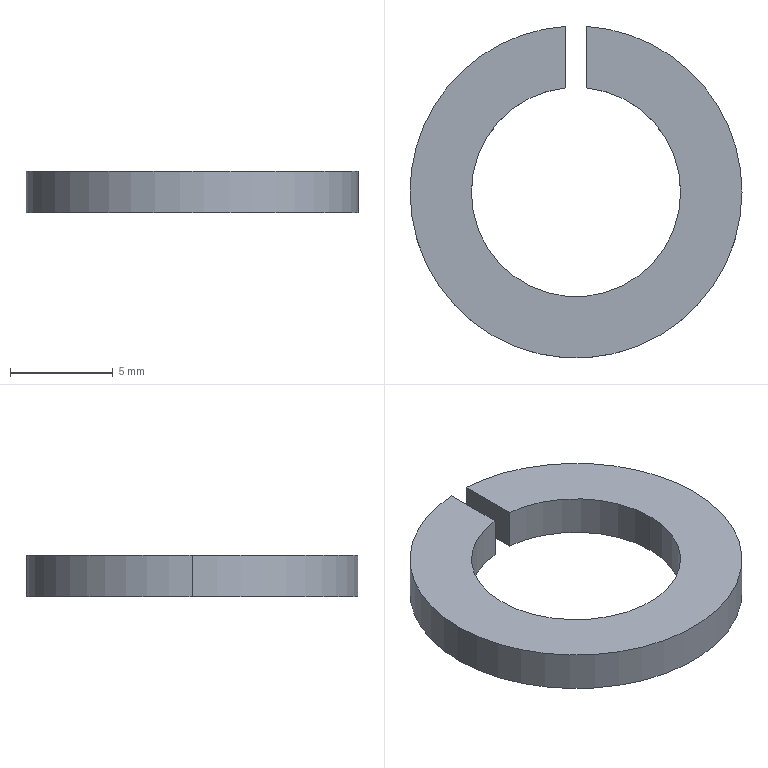Part | SolidWorks | features Extrusion 1 | 1 solid | 10 faces | box 16.182 x 16.166 x 2 mm | volume 241.9 mm3 | cylinder 6 | plane 4 | commonest cylinder face diameters 10.2 x3 16.182 x3
STEP:
#1=CARTESIAN_POINT('',(5.1,0.,2.));
#2=VERTEX_POINT('',#1);
#3=CARTESIAN_POINT('',(-5.1,0.,2.));
#4=VERTEX_POINT('',#3);
#5=CARTESIAN_POINT('',(0.,0.,2.));
#6=DIRECTION('',(0.,0.,-1.));
#7=DIRECTION('',(1.,0.,0.));
#8=AXIS2_PLACEMENT_3D('',#5,#6,#7);
#9=CIRCLE('',#8,5.1);
#10=EDGE_CURVE('',#2,#4,#9,.T.);
#11=ORIENTED_EDGE('',*,*,#10,.F.);
#12=CARTESIAN_POINT('',(5.1,0.,0.));
#13=VERTEX_POINT('',#12);
#14=CARTESIAN_POINT('',(5.1,0.,2.));
#15=DIRECTION('',(0.,0.,-1.));
#16=VECTOR('',#15,1000.);
#17=LINE('',#14,#16);
#18=EDGE_CURVE('',#2,#13,#17,.T.);
#19=ORIENTED_EDGE('',*,*,#18,.T.);
#20=CARTESIAN_POINT('',(-5.1,0.,0.));
#21=VERTEX_POINT('',#20);
#22=CARTESIAN_POINT('',(0.,0.,0.));
#23=DIRECTION('',(0.,0.,-1.));
#24=DIRECTION('',(1.,0.,0.));
#25=AXIS2_PLACEMENT_3D('',#22,#23,#24);
#26=CIRCLE('',#25,5.1);
#27=EDGE_CURVE('',#13,#21,#26,.T.);
#28=ORIENTED_EDGE('',*,*,#27,.T.);
#29=CARTESIAN_POINT('',(-5.1,0.,2.));
#30=DIRECTION('',(0.,0.,-1.));
#31=VECTOR('',#30,1000.);
#32=LINE('',#29,#31);
#33=EDGE_CURVE('',#4,#21,#32,.T.);
#34=ORIENTED_EDGE('',*,*,#33,.F.);
#35=EDGE_LOOP('',(#11,#19,#28,#34));
#36=FACE_OUTER_BOUND('',#35,.T.);
#37=CARTESIAN_POINT('',(0.,0.,2.));
#38=DIRECTION('',(0.,0.,-1.));
#39=DIRECTION('',(-1.,0.,0.));
#40=AXIS2_PLACEMENT_3D('',#37,#38,#39);
#41=CYLINDRICAL_SURFACE('',#40,5.1);
#42=ADVANCED_FACE('',(#36),#41,.F.);
#43=CARTESIAN_POINT('',(-0.5,5.075,2.));
#44=VERTEX_POINT('',#43);
#45=CARTESIAN_POINT('',(0.,0.,2.));
#46=DIRECTION('',(0.,0.,-1.));
#47=DIRECTION('',(1.,0.,0.));
#48=AXIS2_PLACEMENT_3D('',#45,#46,#47);
#49=CIRCLE('',#48,5.1);
#50=EDGE_CURVE('',#4,#44,#49,.T.);
#51=ORIENTED_EDGE('',*,*,#50,.F.);
#52=ORIENTED_EDGE('',*,*,#33,.T.);
#53=CARTESIAN_POINT('',(-0.5,5.075,0.));
#54=VERTEX_POINT('',#53);
#55=CARTESIAN_POINT('',(0.,0.,0.));
#56=DIRECTION('',(0.,0.,-1.));
#57=DIRECTION('',(1.,0.,0.));
#58=AXIS2_PLACEMENT_3D('',#55,#56,#57);
#59=CIRCLE('',#58,5.1);
#60=EDGE_CURVE('',#21,#54,#59,.T.);
#61=ORIENTED_EDGE('',*,*,#60,.T.);
#62=CARTESIAN_POINT('',(-0.5,5.075,2.));
#63=DIRECTION('',(0.,0.,-1.));
#64=VECTOR('',#63,1000.);
#65=LINE('',#62,#64);
#66=EDGE_CURVE('',#44,#54,#65,.T.);
#67=ORIENTED_EDGE('',*,*,#66,.F.);
#68=EDGE_LOOP('',(#51,#52,#61,#67));
#69=FACE_OUTER_BOUND('',#68,.T.);
#70=CARTESIAN_POINT('',(0.,0.,2.));
#71=DIRECTION('',(0.,0.,-1.));
#72=DIRECTION('',(-1.,0.,0.));
#73=AXIS2_PLACEMENT_3D('',#70,#71,#72);
#74=CYLINDRICAL_SURFACE('',#73,5.1);
#75=ADVANCED_FACE('',(#69),#74,.F.);
#76=CARTESIAN_POINT('',(8.091,0.,2.));
#77=VERTEX_POINT('',#76);
#78=CARTESIAN_POINT('',(0.5,8.075,2.));
#79=VERTEX_POINT('',#78);
#80=CARTESIAN_POINT('',(0.,0.,2.));
#81=DIRECTION('',(0.,0.,1.));
#82=DIRECTION('',(1.,0.,0.));
#83=AXIS2_PLACEMENT_3D('',#80,#81,#82);
#84=CIRCLE('',#83,8.091);
#85=EDGE_CURVE('',#77,#79,#84,.T.);
#86=ORIENTED_EDGE('',*,*,#85,.F.);
#87=CARTESIAN_POINT('',(8.091,0.,0.));
#88=VERTEX_POINT('',#87);
#89=CARTESIAN_POINT('',(8.091,0.,2.));
#90=DIRECTION('',(0.,0.,-1.));
#91=VECTOR('',#90,1000.);
#92=LINE('',#89,#91);
#93=EDGE_CURVE('',#77,#88,#92,.T.);
#94=ORIENTED_EDGE('',*,*,#93,.T.);
#95=CARTESIAN_POINT('',(0.5,8.075,0.));
#96=VERTEX_POINT('',#95);
#97=CARTESIAN_POINT('',(0.,0.,0.));
#98=DIRECTION('',(0.,0.,1.));
#99=DIRECTION('',(1.,0.,0.));
#100=AXIS2_PLACEMENT_3D('',#97,#98,#99);
#101=CIRCLE('',#100,8.091);
#102=EDGE_CURVE('',#88,#96,#101,.T.);
#103=ORIENTED_EDGE('',*,*,#102,.T.);
#104=CARTESIAN_POINT('',(0.5,8.075,2.));
#105=DIRECTION('',(0.,0.,-1.));
#106=VECTOR('',#105,1000.);
#107=LINE('',#104,#106);
#108=EDGE_CURVE('',#79,#96,#107,.T.);
#109=ORIENTED_EDGE('',*,*,#108,.F.);
#110=EDGE_LOOP('',(#86,#94,#103,#109));
#111=FACE_OUTER_BOUND('',#110,.T.);
#112=CARTESIAN_POINT('',(0.,0.,2.));
#113=DIRECTION('',(0.,0.,-1.));
#114=DIRECTION('',(-1.,0.,0.));
#115=AXIS2_PLACEMENT_3D('',#112,#113,#114);
#116=CYLINDRICAL_SURFACE('',#115,8.091);
#117=ADVANCED_FACE('',(#111),#116,.T.);
#118=ORIENTED_EDGE('',*,*,#93,.F.);
#119=CARTESIAN_POINT('',(-8.091,0.,2.));
#120=VERTEX_POINT('',#119);
#121=CARTESIAN_POINT('',(0.,0.,2.));
#122=DIRECTION('',(0.,0.,1.));
#123=DIRECTION('',(1.,0.,0.));
#124=AXIS2_PLACEMENT_3D('',#121,#122,#123);
#125=CIRCLE('',#124,8.091);
#126=EDGE_CURVE('',#120,#77,#125,.T.);
#127=ORIENTED_EDGE('',*,*,#126,.F.);
#128=CARTESIAN_POINT('',(-8.091,0.,0.));
#129=VERTEX_POINT('',#128);
#130=CARTESIAN_POINT('',(-8.091,0.,2.));
#131=DIRECTION('',(0.,0.,-1.));
#132=VECTOR('',#131,1000.);
#133=LINE('',#130,#132);
#134=EDGE_CURVE('',#120,#129,#133,.T.);
#135=ORIENTED_EDGE('',*,*,#134,.T.);
#136=CARTESIAN_POINT('',(0.,0.,0.));
#137=DIRECTION('',(0.,0.,1.));
#138=DIRECTION('',(1.,0.,0.));
#139=AXIS2_PLACEMENT_3D('',#136,#137,#138);
#140=CIRCLE('',#139,8.091);
#141=EDGE_CURVE('',#129,#88,#140,.T.);
#142=ORIENTED_EDGE('',*,*,#141,.T.);
#143=EDGE_LOOP('',(#118,#127,#135,#142));
#144=FACE_OUTER_BOUND('',#143,.T.);
#145=CARTESIAN_POINT('',(0.,0.,2.));
#146=DIRECTION('',(0.,0.,-1.));
#147=DIRECTION('',(-1.,0.,0.));
#148=AXIS2_PLACEMENT_3D('',#145,#146,#147);
#149=CYLINDRICAL_SURFACE('',#148,8.091);
#150=ADVANCED_FACE('',(#144),#149,.T.);
#151=ORIENTED_EDGE('',*,*,#134,.F.);
#152=CARTESIAN_POINT('',(-0.5,8.075,2.));
#153=VERTEX_POINT('',#152);
#154=CARTESIAN_POINT('',(0.,0.,2.));
#155=DIRECTION('',(0.,0.,1.));
#156=DIRECTION('',(1.,0.,0.));
#157=AXIS2_PLACEMENT_3D('',#154,#155,#156);
#158=CIRCLE('',#157,8.091);
#159=EDGE_CURVE('',#153,#120,#158,.T.);
#160=ORIENTED_EDGE('',*,*,#159,.F.);
#161=CARTESIAN_POINT('',(-0.5,8.075,0.));
#162=VERTEX_POINT('',#161);
#163=CARTESIAN_POINT('',(-0.5,8.075,2.));
#164=DIRECTION('',(0.,0.,-1.));
#165=VECTOR('',#164,1000.);
#166=LINE('',#163,#165);
#167=EDGE_CURVE('',#153,#162,#166,.T.);
#168=ORIENTED_EDGE('',*,*,#167,.T.);
#169=CARTESIAN_POINT('',(0.,0.,0.));
#170=DIRECTION('',(0.,0.,1.));
#171=DIRECTION('',(1.,0.,0.));
#172=AXIS2_PLACEMENT_3D('',#169,#170,#171);
#173=CIRCLE('',#172,8.091);
#174=EDGE_CURVE('',#162,#129,#173,.T.);
#175=ORIENTED_EDGE('',*,*,#174,.T.);
#176=EDGE_LOOP('',(#151,#160,#168,#175));
#177=FACE_OUTER_BOUND('',#176,.T.);
#178=CARTESIAN_POINT('',(0.,0.,2.));
#179=DIRECTION('',(0.,0.,-1.));
#180=DIRECTION('',(-1.,0.,0.));
#181=AXIS2_PLACEMENT_3D('',#178,#179,#180);
#182=CYLINDRICAL_SURFACE('',#181,8.091);
#183=ADVANCED_FACE('',(#177),#182,.T.);
#184=CARTESIAN_POINT('',(0.5,5.075,0.));
#185=VERTEX_POINT('',#184);
#186=CARTESIAN_POINT('',(0.5,8.075,0.));
#187=DIRECTION('',(0.,-1.,0.));
#188=VECTOR('',#187,1000.);
#189=LINE('',#186,#188);
#190=EDGE_CURVE('',#96,#185,#189,.T.);
#191=ORIENTED_EDGE('',*,*,#190,.T.);
#192=CARTESIAN_POINT('',(0.5,5.075,2.));
#193=VERTEX_POINT('',#192);
#194=CARTESIAN_POINT('',(0.5,5.075,2.));
#195=DIRECTION('',(0.,0.,-1.));
#196=VECTOR('',#195,1000.);
#197=LINE('',#194,#196);
#198=EDGE_CURVE('',#193,#185,#197,.T.);
#199=ORIENTED_EDGE('',*,*,#198,.F.);
#200=CARTESIAN_POINT('',(0.5,8.075,2.));
#201=DIRECTION('',(0.,-1.,0.));
#202=VECTOR('',#201,1000.);
#203=LINE('',#200,#202);
#204=EDGE_CURVE('',#79,#193,#203,.T.);
#205=ORIENTED_EDGE('',*,*,#204,.F.);
#206=ORIENTED_EDGE('',*,*,#108,.T.);
#207=EDGE_LOOP('',(#191,#199,#205,#206));
#208=FACE_OUTER_BOUND('',#207,.T.);
#209=CARTESIAN_POINT('',(0.5,8.075,2.));
#210=DIRECTION('',(1.,0.,0.));
#211=DIRECTION('',(0.,1.,0.));
#212=AXIS2_PLACEMENT_3D('',#209,#210,#211);
#213=PLANE('',#212);
#214=ADVANCED_FACE('',(#208),#213,.F.);
#215=ORIENTED_EDGE('',*,*,#18,.F.);
#216=CARTESIAN_POINT('',(0.,0.,2.));
#217=DIRECTION('',(0.,0.,-1.));
#218=DIRECTION('',(1.,0.,0.));
#219=AXIS2_PLACEMENT_3D('',#216,#217,#218);
#220=CIRCLE('',#219,5.1);
#221=EDGE_CURVE('',#193,#2,#220,.T.);
#222=ORIENTED_EDGE('',*,*,#221,.F.);
#223=ORIENTED_EDGE('',*,*,#198,.T.);
#224=CARTESIAN_POINT('',(0.,0.,0.));
#225=DIRECTION('',(0.,0.,-1.));
#226=DIRECTION('',(1.,0.,0.));
#227=AXIS2_PLACEMENT_3D('',#224,#225,#226);
#228=CIRCLE('',#227,5.1);
#229=EDGE_CURVE('',#185,#13,#228,.T.);
#230=ORIENTED_EDGE('',*,*,#229,.T.);
#231=EDGE_LOOP('',(#215,#222,#223,#230));
#232=FACE_OUTER_BOUND('',#231,.T.);
#233=CARTESIAN_POINT('',(0.,0.,2.));
#234=DIRECTION('',(0.,0.,-1.));
#235=DIRECTION('',(-1.,0.,0.));
#236=AXIS2_PLACEMENT_3D('',#233,#234,#235);
#237=CYLINDRICAL_SURFACE('',#236,5.1);
#238=ADVANCED_FACE('',(#232),#237,.F.);
#239=CARTESIAN_POINT('',(-0.5,8.075,0.));
#240=DIRECTION('',(0.,1.,0.));
#241=VECTOR('',#240,1000.);
#242=LINE('',#239,#241);
#243=EDGE_CURVE('',#54,#162,#242,.T.);
#244=ORIENTED_EDGE('',*,*,#243,.T.);
#245=ORIENTED_EDGE('',*,*,#167,.F.);
#246=CARTESIAN_POINT('',(-0.5,8.075,2.));
#247=DIRECTION('',(0.,1.,0.));
#248=VECTOR('',#247,1000.);
#249=LINE('',#246,#248);
#250=EDGE_CURVE('',#44,#153,#249,.T.);
#251=ORIENTED_EDGE('',*,*,#250,.F.);
#252=ORIENTED_EDGE('',*,*,#66,.T.);
#253=EDGE_LOOP('',(#244,#245,#251,#252));
#254=FACE_OUTER_BOUND('',#253,.T.);
#255=CARTESIAN_POINT('',(-0.5,8.075,2.));
#256=DIRECTION('',(-1.,0.,0.));
#257=DIRECTION('',(0.,-1.,0.));
#258=AXIS2_PLACEMENT_3D('',#255,#256,#257);
#259=PLANE('',#258);
#260=ADVANCED_FACE('',(#254),#259,.F.);
#261=ORIENTED_EDGE('',*,*,#159,.T.);
#262=ORIENTED_EDGE('',*,*,#126,.T.);
#263=ORIENTED_EDGE('',*,*,#85,.T.);
#264=ORIENTED_EDGE('',*,*,#204,.T.);
#265=ORIENTED_EDGE('',*,*,#221,.T.);
#266=ORIENTED_EDGE('',*,*,#10,.T.);
#267=ORIENTED_EDGE('',*,*,#50,.T.);
#268=ORIENTED_EDGE('',*,*,#250,.T.);
#269=EDGE_LOOP('',(#261,#262,#263,#264,#265,#266,#267,#268));
#270=FACE_OUTER_BOUND('',#269,.T.);
#271=CARTESIAN_POINT('',(0.,0.,2.));
#272=DIRECTION('',(0.,0.,1.));
#273=DIRECTION('',(1.,0.,0.));
#274=AXIS2_PLACEMENT_3D('',#271,#272,#273);
#275=PLANE('',#274);
#276=ADVANCED_FACE('',(#270),#275,.T.);
#277=ORIENTED_EDGE('',*,*,#174,.F.);
#278=ORIENTED_EDGE('',*,*,#243,.F.);
#279=ORIENTED_EDGE('',*,*,#60,.F.);
#280=ORIENTED_EDGE('',*,*,#27,.F.);
#281=ORIENTED_EDGE('',*,*,#229,.F.);
#282=ORIENTED_EDGE('',*,*,#190,.F.);
#283=ORIENTED_EDGE('',*,*,#102,.F.);
#284=ORIENTED_EDGE('',*,*,#141,.F.);
#285=EDGE_LOOP('',(#277,#278,#279,#280,#281,#282,#283,#284));
#286=FACE_OUTER_BOUND('',#285,.T.);
#287=CARTESIAN_POINT('',(0.,0.,0.));
#288=DIRECTION('',(0.,0.,1.));
#289=DIRECTION('',(1.,0.,0.));
#290=AXIS2_PLACEMENT_3D('',#287,#288,#289);
#291=PLANE('',#290);
#292=ADVANCED_FACE('',(#286),#291,.F.);
#293=CLOSED_SHELL('',(#42,#75,#117,#150,#183,#214,#238,#260,#276,#292));
#294=MANIFOLD_SOLID_BREP('',#293);
#295=CARTESIAN_POINT('',(0.,0.,0.));
#296=DIRECTION('',(0.,0.,1.));
#297=DIRECTION('',(1.,0.,0.));
#298=AXIS2_PLACEMENT_3D('',#295,#296,#297);
#299=(LENGTH_UNIT()NAMED_UNIT(*)SI_UNIT(.MILLI.,.METRE.));
#300=UNCERTAINTY_MEASURE_WITH_UNIT(LENGTH_MEASURE(0.00001),#299,'','');
#301=(NAMED_UNIT(*)PLANE_ANGLE_UNIT()SI_UNIT($,.RADIAN.));
#302=(NAMED_UNIT(*)SI_UNIT($,.STERADIAN.)SOLID_ANGLE_UNIT());
#303=(GEOMETRIC_REPRESENTATION_CONTEXT(3)GLOBAL_UNCERTAINTY_ASSIGNED_CONTEXT((#300))GLOBAL_UNIT_ASSIGNED_CONTEXT((#299,#301,#302))REPRESENTATION_CONTEXT('',''));
#304=ADVANCED_BREP_SHAPE_REPRESENTATION('',(#294,#298),#303);